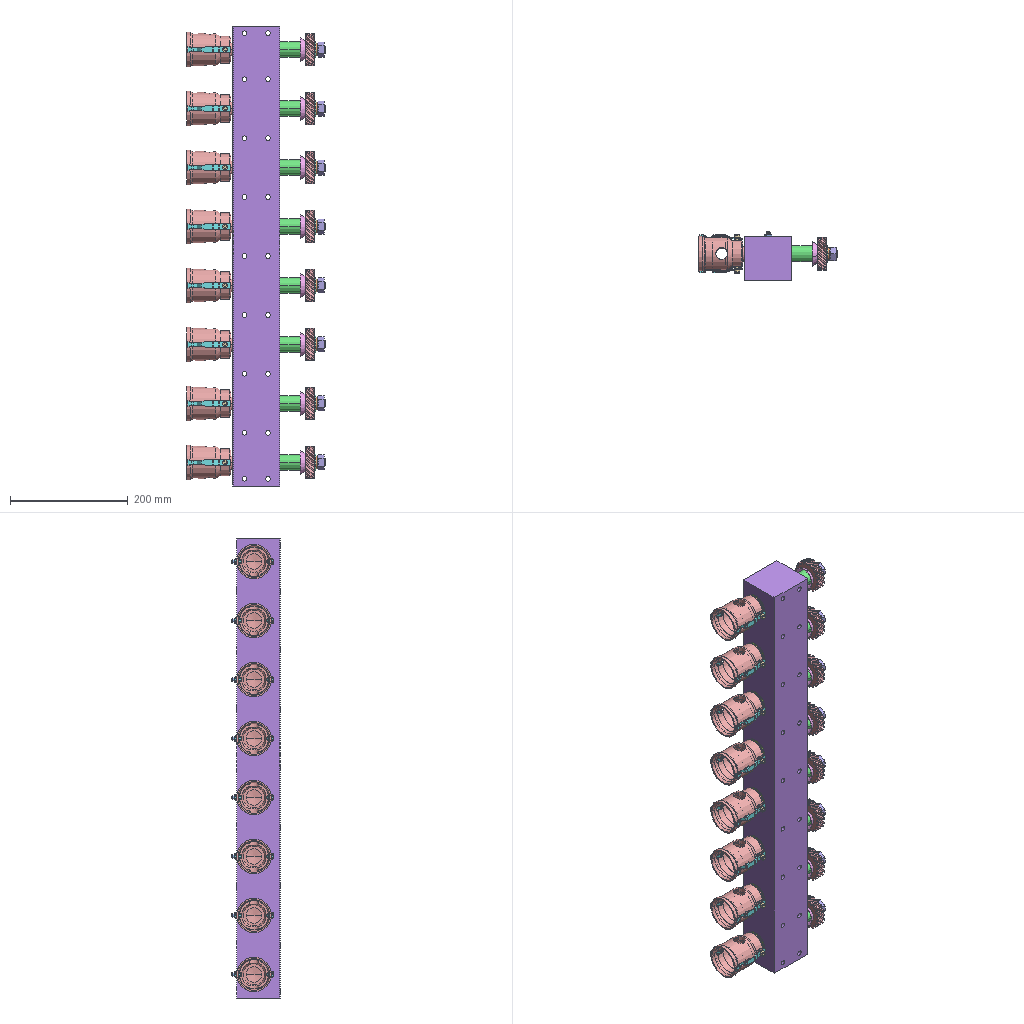Assembly | SolidWorks | 14 different items | 129 placed | box 235 x 83 x 780 mm
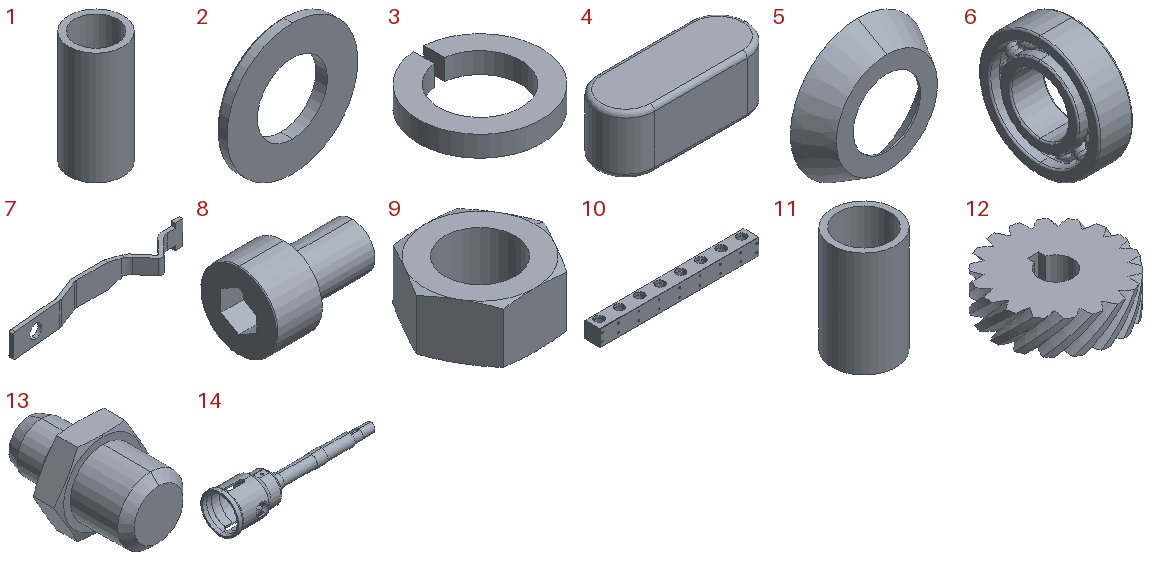Parts list (item | quantity | size | volume | features):
1 | x8 | 27 x 27 x 56 mm | 12667 mm3 | features Extrusion 1
2 | x8 | 28 x 2.5 x 28 mm | 1081 mm3 | features Revolution 1
3 | x8 | 21.361 x 21.323 x 3.6 mm | 696.819 mm3 | features Extrusion 1
4 | x8 | 13 x 5 x 5 mm | 296.036 mm3 | features Extrusion 1, Fillet 1
5 | x8 | 40 x 8.91 x 40 mm | 725.876 mm3 | features Revolution 1
6 | x16 | 12 x 42 x 42 mm | 9401 mm3 | features Revolution 4, CirPattern 2, RefAxis 1, RevCut 1
7 | x16 | 73 x 9 x 9.5 mm | 954.396 mm3 | features Extrusion 1, ICE 1
8 | x16 | 13 x 8.5 x 8.5 mm | 404.848 mm3 | features BlendCut 1, Cut 1, Fillet 1, LPattern 1, RevCut 1, Revolution 1
9 | x8 | 25.4 x 21.997 x 11 mm | 2905 mm3 | features Cut 2, Chamfer 1, Extrusion 1
10 | x1 | 780 x 74 x 80 mm | 3762730 mm3 | features MirrorPattern 4, HoleWzd 3, LPattern 3, Chamfer 2, ICE 2, Extrusion 1
11 | x8 | 26 x 26 x 43 mm | 7936 mm3 | features ICE 1, LibraryFeature 1
12 | x8 | 54.912 x 54.912 x 15 mm | 29067 mm3 | features ICE 2, CirPattern 1, Extrusion 1, Helix 1, RefAxis 1, SweepCut 1
13 | x8 | 11.547 x 15.8 x 10 mm | 760.457 mm3 | features RevCut 2, Chamfer 1, Extrusion 1, ICE 1, Revolution 1
14 | x8 | 235 x 59 x 59 mm | 87330 mm3 | features ICE 4, MirrorPattern 1, Revolution 1
Mates (type | each side: item.copy, entity, surface, feature):
Concentric | 14.1 face cylinder Revolve1 | 6.1 face cylinder Revolve1
Coincident | 14.1 face plane Revolve1 | 6.1 face plane Revolve1
DistanceDim | 14.1 face plane Cut-Extrude1 | 7.1 face plane Cut-Extrude1
DistanceDim | 7.1 face plane Boss-Extrude1 | 14.1 face plane Cut-Extrude2
DistanceDim | 7.1 face plane Boss-Extrude1 | 14.1 face plane Revolve1
DistanceDim | 7.2 face plane Boss-Extrude1 | 14.1 face plane Revolve1
DistanceDim | 7.2 face plane Boss-Extrude1 | 14.1 face plane Mirror1
DistanceDim | 7.2 face plane Cut-Extrude1 | 14.1 face plane Cut-Extrude1
Concentric | 14.1 face cylinder Cut-Extrude1 | 8.1 face cylinder Base-Revolve
DistanceDim | 8.1 face plane Base-Revolve | 14.1 face plane Mirror1
DistanceDim | 8.2 face plane Base-Revolve | 14.1 face plane Cut-Extrude2
Concentric | 14.1 face cylinder Cut-Extrude1 | 8.2 face cylinder Base-Revolve
Concentric | 6.2 face cylinder Revolve1 | 10.1 face cylinder Mirror1
Concentric | 6.1 face cylinder Revolve1 | 10.1 face cylinder Cut-Extrude1
Coincident | 6.1 face plane Revolve1 | 10.1 face plane Cut-Extrude1
Coincident | 6.2 face plane Revolve1 | 10.1 face plane Mirror1
Concentric | 14.1 face cylinder Revolve1 | 11.1 face cylinder Boss-Extrude1
Coincident | 6.2 face plane Revolve1 | 11.1 face plane Boss-Extrude1
Concentric | 14.1 face cylinder Revolve1 | 12.1 face cylinder Cut-Extrude1
Parallel | 7.2 face plane Boss-Extrude1 | 10.1 face plane Boss-Extrude1
Concentric | 10.1 face cylinder M8 Tapped Hole1 | 13.1 face cylinder Boss-Extrude1
Coincident | 10.1 face plane Boss-Extrude1 | 13.1 face plane Boss-Extrude2
Concentric | 14.1 face cylinder Revolve1 | 1.1 face cylinder Boss-Extrude1
Coincident | 6.2 face plane Revolve1 | 1.1 face plane Boss-Extrude1
Coincident | 11.1 face plane Boss-Extrude1 | 5.1 face plane Revolve1
Concentric | 14.1 face cylinder Revolve1 | 5.1 face cylinder Revolve1
Coincident | 12.1 face plane Boss-Extrude1 | 5.1 face plane Revolve1
Concentric | 14.1 edge | 2.1 face cylinder Base-Revolve
Coincident | 12.1 face plane Boss-Extrude1 | 2.1 face plane Base-Revolve
Concentric | 14.1 face cylinder Revolve1 | 3.1 face cylinder Extrude1
Coincident | 2.1 face plane Base-Revolve | 3.1 face plane Extrude1
Concentric | 14.1 face cylinder Revolve1 | 9.1 face cylinder Base-Extrude
Coincident | 3.1 face plane Extrude1 | 9.1 face plane Base-Extrude
Coincident | 14.1 face plane Cut-Extrude4 | 4.1 face plane Base-Extrude | 2 times